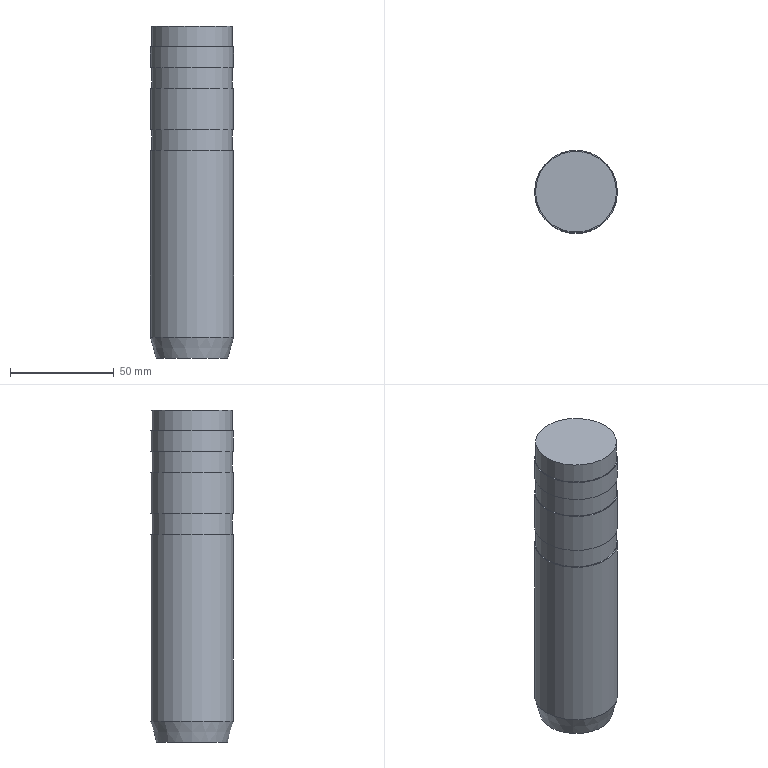Part | NX | features solid 2 | 1 solid | 14 faces | box 40 x 40 x 160 mm | volume 197592 mm3 | plane 7 | cylinder 6 | cone 1 | commonest cylinder face diameters 39 x3 40 x3
STEP:
#1=CARTESIAN_POINT('',(-324.5,-10.,105.));
#2=VERTEX_POINT('',#1);
#3=CARTESIAN_POINT('',(-305.,-10.,105.));
#4=DIRECTION('',(0.,0.,-1.));
#5=DIRECTION('',(-1.,0.,0.));
#6=AXIS2_PLACEMENT_3D('',#3,#4,#5);
#7=CIRCLE('',#6,19.5);
#8=EDGE_CURVE('',#2,#2,#7,.T.);
#9=ORIENTED_EDGE('',*,*,#8,.F.);
#10=EDGE_LOOP('',(#9));
#11=FACE_BOUND('',#10,.T.);
#12=CARTESIAN_POINT('',(-324.5,-10.,115.));
#13=VERTEX_POINT('',#12);
#14=CARTESIAN_POINT('',(-305.,-10.,115.));
#15=DIRECTION('',(0.,0.,-1.));
#16=DIRECTION('',(-1.,0.,0.));
#17=AXIS2_PLACEMENT_3D('',#14,#15,#16);
#18=CIRCLE('',#17,19.5);
#19=EDGE_CURVE('',#13,#13,#18,.T.);
#20=ORIENTED_EDGE('',*,*,#19,.T.);
#21=EDGE_LOOP('',(#20));
#22=FACE_BOUND('',#21,.T.);
#23=CARTESIAN_POINT('',(-305.,-10.,105.));
#24=DIRECTION('',(0.,0.,1.));
#25=DIRECTION('',(1.,0.,0.));
#26=AXIS2_PLACEMENT_3D('',#23,#24,#25);
#27=CYLINDRICAL_SURFACE('',#26,19.5);
#28=ADVANCED_FACE('',(#11,#22),#27,.T.);
#29=CARTESIAN_POINT('',(-325.,-10.,105.));
#30=VERTEX_POINT('',#29);
#31=CARTESIAN_POINT('',(-305.,-10.,105.));
#32=DIRECTION('',(0.,0.,-1.));
#33=DIRECTION('',(-1.,0.,0.));
#34=AXIS2_PLACEMENT_3D('',#31,#32,#33);
#35=CIRCLE('',#34,20.);
#36=EDGE_CURVE('',#30,#30,#35,.T.);
#37=ORIENTED_EDGE('',*,*,#36,.F.);
#38=EDGE_LOOP('',(#37));
#39=FACE_BOUND('',#38,.T.);
#40=ORIENTED_EDGE('',*,*,#8,.T.);
#41=EDGE_LOOP('',(#40));
#42=FACE_BOUND('',#41,.T.);
#43=CARTESIAN_POINT('',(-305.,-10.,105.));
#44=DIRECTION('',(0.,0.,-1.));
#45=DIRECTION('',(-1.,0.,0.));
#46=AXIS2_PLACEMENT_3D('',#43,#44,#45);
#47=PLANE('',#46);
#48=ADVANCED_FACE('',(#39,#42),#47,.F.);
#49=CARTESIAN_POINT('',(-325.,-10.,15.));
#50=VERTEX_POINT('',#49);
#51=CARTESIAN_POINT('',(-305.,-10.,15.));
#52=DIRECTION('',(0.,0.,-1.));
#53=DIRECTION('',(-1.,0.,0.));
#54=AXIS2_PLACEMENT_3D('',#51,#52,#53);
#55=CIRCLE('',#54,20.);
#56=EDGE_CURVE('',#50,#50,#55,.T.);
#57=ORIENTED_EDGE('',*,*,#56,.F.);
#58=EDGE_LOOP('',(#57));
#59=FACE_BOUND('',#58,.T.);
#60=ORIENTED_EDGE('',*,*,#36,.T.);
#61=EDGE_LOOP('',(#60));
#62=FACE_BOUND('',#61,.T.);
#63=CARTESIAN_POINT('',(-305.,-10.,55.));
#64=DIRECTION('',(0.,0.,1.));
#65=DIRECTION('',(1.,0.,0.));
#66=AXIS2_PLACEMENT_3D('',#63,#64,#65);
#67=CYLINDRICAL_SURFACE('',#66,20.);
#68=ADVANCED_FACE('',(#59,#62),#67,.T.);
#69=CARTESIAN_POINT('',(-322.321,-10.,5.));
#70=VERTEX_POINT('',#69);
#71=CARTESIAN_POINT('',(-305.,-10.,5.));
#72=DIRECTION('',(0.,0.,-1.));
#73=DIRECTION('',(-1.,0.,0.));
#74=AXIS2_PLACEMENT_3D('',#71,#72,#73);
#75=CIRCLE('',#74,17.321);
#76=EDGE_CURVE('',#70,#70,#75,.T.);
#77=ORIENTED_EDGE('',*,*,#76,.F.);
#78=EDGE_LOOP('',(#77));
#79=FACE_BOUND('',#78,.T.);
#80=ORIENTED_EDGE('',*,*,#56,.T.);
#81=EDGE_LOOP('',(#80));
#82=FACE_BOUND('',#81,.T.);
#83=CARTESIAN_POINT('',(-305.,-10.,15.));
#84=DIRECTION('',(0.,0.,1.));
#85=DIRECTION('',(-1.,0.,0.));
#86=AXIS2_PLACEMENT_3D('',#83,#84,#85);
#87=CONICAL_SURFACE('',#86,20.,0.2618);
#88=ADVANCED_FACE('',(#79,#82),#87,.T.);
#89=ORIENTED_EDGE('',*,*,#76,.T.);
#90=EDGE_LOOP('',(#89));
#91=FACE_BOUND('',#90,.T.);
#92=CARTESIAN_POINT('',(-305.,-10.,5.));
#93=DIRECTION('',(0.,0.,-1.));
#94=DIRECTION('',(-1.,0.,0.));
#95=AXIS2_PLACEMENT_3D('',#92,#93,#94);
#96=PLANE('',#95);
#97=ADVANCED_FACE('',(#91),#96,.T.);
#98=CARTESIAN_POINT('',(-325.,-10.,115.));
#99=VERTEX_POINT('',#98);
#100=CARTESIAN_POINT('',(-305.,-10.,115.));
#101=DIRECTION('',(0.,0.,-1.));
#102=DIRECTION('',(-1.,0.,0.));
#103=AXIS2_PLACEMENT_3D('',#100,#101,#102);
#104=CIRCLE('',#103,20.);
#105=EDGE_CURVE('',#99,#99,#104,.T.);
#106=ORIENTED_EDGE('',*,*,#105,.T.);
#107=EDGE_LOOP('',(#106));
#108=FACE_BOUND('',#107,.T.);
#109=ORIENTED_EDGE('',*,*,#19,.F.);
#110=EDGE_LOOP('',(#109));
#111=FACE_BOUND('',#110,.T.);
#112=CARTESIAN_POINT('',(-305.,-10.,115.));
#113=DIRECTION('',(0.,0.,-1.));
#114=DIRECTION('',(-1.,0.,0.));
#115=AXIS2_PLACEMENT_3D('',#112,#113,#114);
#116=PLANE('',#115);
#117=ADVANCED_FACE('',(#108,#111),#116,.T.);
#118=CARTESIAN_POINT('',(-325.,-10.,135.));
#119=VERTEX_POINT('',#118);
#120=CARTESIAN_POINT('',(-305.,-10.,135.));
#121=DIRECTION('',(0.,0.,-1.));
#122=DIRECTION('',(-1.,0.,0.));
#123=AXIS2_PLACEMENT_3D('',#120,#121,#122);
#124=CIRCLE('',#123,20.);
#125=EDGE_CURVE('',#119,#119,#124,.T.);
#126=ORIENTED_EDGE('',*,*,#125,.T.);
#127=EDGE_LOOP('',(#126));
#128=FACE_BOUND('',#127,.T.);
#129=ORIENTED_EDGE('',*,*,#105,.F.);
#130=EDGE_LOOP('',(#129));
#131=FACE_BOUND('',#130,.T.);
#132=CARTESIAN_POINT('',(-305.,-10.,135.));
#133=DIRECTION('',(0.,0.,-1.));
#134=DIRECTION('',(-1.,0.,0.));
#135=AXIS2_PLACEMENT_3D('',#132,#133,#134);
#136=CYLINDRICAL_SURFACE('',#135,20.);
#137=ADVANCED_FACE('',(#128,#131),#136,.T.);
#138=CARTESIAN_POINT('',(-324.5,-10.,135.));
#139=VERTEX_POINT('',#138);
#140=CARTESIAN_POINT('',(-305.,-10.,135.));
#141=DIRECTION('',(0.,0.,-1.));
#142=DIRECTION('',(-1.,0.,0.));
#143=AXIS2_PLACEMENT_3D('',#140,#141,#142);
#144=CIRCLE('',#143,19.5);
#145=EDGE_CURVE('',#139,#139,#144,.T.);
#146=ORIENTED_EDGE('',*,*,#145,.T.);
#147=EDGE_LOOP('',(#146));
#148=FACE_BOUND('',#147,.T.);
#149=ORIENTED_EDGE('',*,*,#125,.F.);
#150=EDGE_LOOP('',(#149));
#151=FACE_BOUND('',#150,.T.);
#152=CARTESIAN_POINT('',(-305.,-10.,135.));
#153=DIRECTION('',(0.,0.,-1.));
#154=DIRECTION('',(-1.,0.,0.));
#155=AXIS2_PLACEMENT_3D('',#152,#153,#154);
#156=PLANE('',#155);
#157=ADVANCED_FACE('',(#148,#151),#156,.F.);
#158=CARTESIAN_POINT('',(-324.5,-10.,145.));
#159=VERTEX_POINT('',#158);
#160=CARTESIAN_POINT('',(-305.,-10.,145.));
#161=DIRECTION('',(0.,0.,-1.));
#162=DIRECTION('',(-1.,0.,0.));
#163=AXIS2_PLACEMENT_3D('',#160,#161,#162);
#164=CIRCLE('',#163,19.5);
#165=EDGE_CURVE('',#159,#159,#164,.F.);
#166=ORIENTED_EDGE('',*,*,#165,.F.);
#167=EDGE_LOOP('',(#166));
#168=FACE_BOUND('',#167,.T.);
#169=ORIENTED_EDGE('',*,*,#145,.F.);
#170=EDGE_LOOP('',(#169));
#171=FACE_BOUND('',#170,.T.);
#172=CARTESIAN_POINT('',(-305.,-10.,145.));
#173=DIRECTION('',(0.,0.,-1.));
#174=DIRECTION('',(-1.,0.,0.));
#175=AXIS2_PLACEMENT_3D('',#172,#173,#174);
#176=CYLINDRICAL_SURFACE('',#175,19.5);
#177=ADVANCED_FACE('',(#168,#171),#176,.T.);
#178=CARTESIAN_POINT('',(-325.,-10.,155.));
#179=VERTEX_POINT('',#178);
#180=CARTESIAN_POINT('',(-305.,-10.,155.));
#181=DIRECTION('',(0.,0.,-1.));
#182=DIRECTION('',(-1.,0.,0.));
#183=AXIS2_PLACEMENT_3D('',#180,#181,#182);
#184=CIRCLE('',#183,20.);
#185=EDGE_CURVE('',#179,#179,#184,.T.);
#186=ORIENTED_EDGE('',*,*,#185,.T.);
#187=EDGE_LOOP('',(#186));
#188=FACE_BOUND('',#187,.T.);
#189=CARTESIAN_POINT('',(-325.,-10.,145.));
#190=VERTEX_POINT('',#189);
#191=CARTESIAN_POINT('',(-305.,-10.,145.));
#192=DIRECTION('',(0.,0.,-1.));
#193=DIRECTION('',(-1.,0.,0.));
#194=AXIS2_PLACEMENT_3D('',#191,#192,#193);
#195=CIRCLE('',#194,20.);
#196=EDGE_CURVE('',#190,#190,#195,.T.);
#197=ORIENTED_EDGE('',*,*,#196,.F.);
#198=EDGE_LOOP('',(#197));
#199=FACE_BOUND('',#198,.T.);
#200=CARTESIAN_POINT('',(-305.,-10.,155.));
#201=DIRECTION('',(0.,0.,-1.));
#202=DIRECTION('',(-1.,0.,0.));
#203=AXIS2_PLACEMENT_3D('',#200,#201,#202);
#204=CYLINDRICAL_SURFACE('',#203,20.);
#205=ADVANCED_FACE('',(#188,#199),#204,.T.);
#206=CARTESIAN_POINT('',(-324.5,-10.,155.));
#207=VERTEX_POINT('',#206);
#208=CARTESIAN_POINT('',(-305.,-10.,155.));
#209=DIRECTION('',(0.,0.,-1.));
#210=DIRECTION('',(-1.,0.,0.));
#211=AXIS2_PLACEMENT_3D('',#208,#209,#210);
#212=CIRCLE('',#211,19.5);
#213=EDGE_CURVE('',#207,#207,#212,.T.);
#214=ORIENTED_EDGE('',*,*,#213,.T.);
#215=EDGE_LOOP('',(#214));
#216=FACE_BOUND('',#215,.T.);
#217=ORIENTED_EDGE('',*,*,#185,.F.);
#218=EDGE_LOOP('',(#217));
#219=FACE_BOUND('',#218,.T.);
#220=CARTESIAN_POINT('',(-305.,-10.,155.));
#221=DIRECTION('',(0.,0.,-1.));
#222=DIRECTION('',(-1.,0.,0.));
#223=AXIS2_PLACEMENT_3D('',#220,#221,#222);
#224=PLANE('',#223);
#225=ADVANCED_FACE('',(#216,#219),#224,.F.);
#226=ORIENTED_EDGE('',*,*,#165,.T.);
#227=EDGE_LOOP('',(#226));
#228=FACE_BOUND('',#227,.T.);
#229=ORIENTED_EDGE('',*,*,#196,.T.);
#230=EDGE_LOOP('',(#229));
#231=FACE_BOUND('',#230,.T.);
#232=CARTESIAN_POINT('',(-305.,-10.,145.));
#233=DIRECTION('',(0.,0.,-1.));
#234=DIRECTION('',(-1.,0.,0.));
#235=AXIS2_PLACEMENT_3D('',#232,#233,#234);
#236=PLANE('',#235);
#237=ADVANCED_FACE('',(#228,#231),#236,.T.);
#238=CARTESIAN_POINT('',(-324.5,-10.,165.));
#239=VERTEX_POINT('',#238);
#240=CARTESIAN_POINT('',(-305.,-10.,165.));
#241=DIRECTION('',(0.,0.,-1.));
#242=DIRECTION('',(-1.,0.,0.));
#243=AXIS2_PLACEMENT_3D('',#240,#241,#242);
#244=CIRCLE('',#243,19.5);
#245=EDGE_CURVE('',#239,#239,#244,.T.);
#246=ORIENTED_EDGE('',*,*,#245,.T.);
#247=EDGE_LOOP('',(#246));
#248=FACE_BOUND('',#247,.T.);
#249=ORIENTED_EDGE('',*,*,#213,.F.);
#250=EDGE_LOOP('',(#249));
#251=FACE_BOUND('',#250,.T.);
#252=CARTESIAN_POINT('',(-305.,-10.,165.));
#253=DIRECTION('',(0.,0.,-1.));
#254=DIRECTION('',(-1.,0.,0.));
#255=AXIS2_PLACEMENT_3D('',#252,#253,#254);
#256=CYLINDRICAL_SURFACE('',#255,19.5);
#257=ADVANCED_FACE('',(#248,#251),#256,.T.);
#258=ORIENTED_EDGE('',*,*,#245,.F.);
#259=EDGE_LOOP('',(#258));
#260=FACE_BOUND('',#259,.T.);
#261=CARTESIAN_POINT('',(-305.,-10.,165.));
#262=DIRECTION('',(0.,0.,-1.));
#263=DIRECTION('',(-1.,0.,0.));
#264=AXIS2_PLACEMENT_3D('',#261,#262,#263);
#265=PLANE('',#264);
#266=ADVANCED_FACE('',(#260),#265,.F.);
#267=CLOSED_SHELL('',(#28,#48,#68,#88,#97,#117,#137,#157,#177,#205,#225,#237,#257,#266));
#268=MANIFOLD_SOLID_BREP('',#267);
#269=(LENGTH_UNIT()NAMED_UNIT(*)SI_UNIT(.MILLI.,.METRE.));
#270=UNCERTAINTY_MEASURE_WITH_UNIT(LENGTH_MEASURE(0.00001),#269,'','');
#271=(NAMED_UNIT(*)PLANE_ANGLE_UNIT()SI_UNIT($,.RADIAN.));
#272=(NAMED_UNIT(*)SI_UNIT($,.STERADIAN.)SOLID_ANGLE_UNIT());
#273=(GEOMETRIC_REPRESENTATION_CONTEXT(3)GLOBAL_UNCERTAINTY_ASSIGNED_CONTEXT((#270))GLOBAL_UNIT_ASSIGNED_CONTEXT((#269,#271,#272))REPRESENTATION_CONTEXT('',''));
#274=ADVANCED_BREP_SHAPE_REPRESENTATION('',(#268),#273);